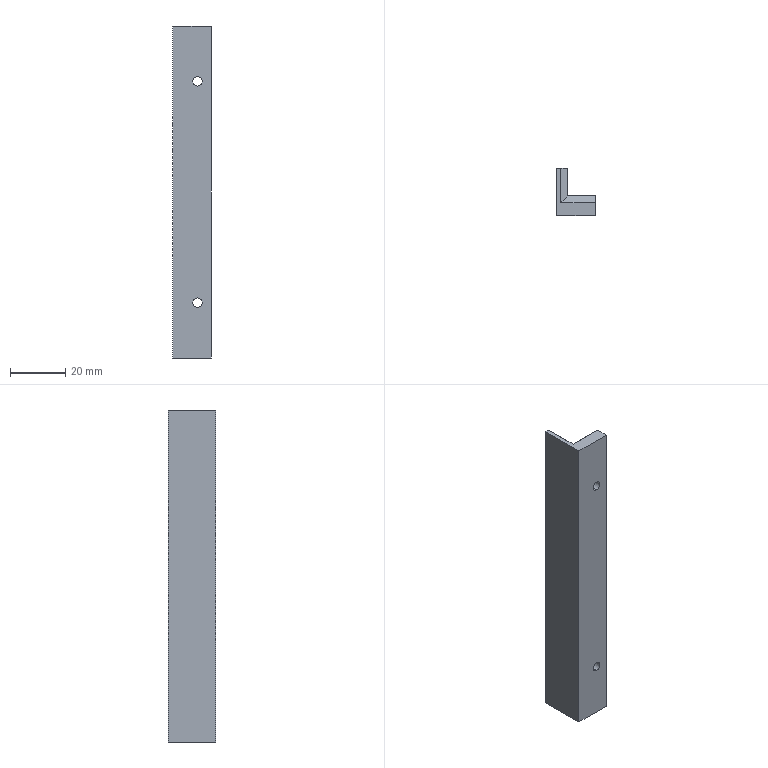Part | NX | features BREP 1 | 1 solid | 20 faces | box 14 x 17 x 120 mm | volume 16235 mm3 | plane 12 | cone 4 | cylinder 4 | commonest cylinder face diameters 3.4 x4
STEP:
#1=CARTESIAN_POINT('',(0.,7.,57.5));
#2=VERTEX_POINT('',#1);
#3=CARTESIAN_POINT('',(0.,4.5,60.));
#4=VERTEX_POINT('',#3);
#5=CARTESIAN_POINT('',(0.,4.5,60.));
#6=DIRECTION('',(0.,-0.7071,0.7071));
#7=VECTOR('',#6,1000.);
#8=LINE('',#5,#7);
#9=EDGE_CURVE('',#2,#4,#8,.T.);
#10=ORIENTED_EDGE('',*,*,#9,.F.);
#11=CARTESIAN_POINT('',(-10.,7.,57.5));
#12=VERTEX_POINT('',#11);
#13=CARTESIAN_POINT('',(-10.,7.,57.5));
#14=DIRECTION('',(1.,0.,0.));
#15=VECTOR('',#14,1000.);
#16=LINE('',#13,#15);
#17=EDGE_CURVE('',#12,#2,#16,.T.);
#18=ORIENTED_EDGE('',*,*,#17,.F.);
#19=CARTESIAN_POINT('',(-12.5,4.5,60.));
#20=VERTEX_POINT('',#19);
#21=CARTESIAN_POINT('',(-8.333,8.667,55.833));
#22=DIRECTION('',(-0.5774,-0.5774,0.5774));
#23=VECTOR('',#22,1000.);
#24=LINE('',#21,#23);
#25=EDGE_CURVE('',#12,#20,#24,.T.);
#26=ORIENTED_EDGE('',*,*,#25,.T.);
#27=CARTESIAN_POINT('',(0.,4.5,60.));
#28=DIRECTION('',(-1.,0.,0.));
#29=VECTOR('',#28,1000.);
#30=LINE('',#27,#29);
#31=EDGE_CURVE('',#4,#20,#30,.T.);
#32=ORIENTED_EDGE('',*,*,#31,.F.);
#33=EDGE_LOOP('',(#10,#18,#26,#32));
#34=FACE_BOUND('',#33,.T.);
#35=CARTESIAN_POINT('',(0.,4.5,60.));
#36=DIRECTION('',(0.,-0.7071,-0.7071));
#37=DIRECTION('',(-1.,0.,0.));
#38=AXIS2_PLACEMENT_3D('',#35,#36,#37);
#39=PLANE('',#38);
#40=ADVANCED_FACE('',(#34),#39,.F.);
#41=CARTESIAN_POINT('',(-12.5,17.,60.));
#42=VERTEX_POINT('',#41);
#43=CARTESIAN_POINT('',(-10.,17.,57.5));
#44=VERTEX_POINT('',#43);
#45=CARTESIAN_POINT('',(-12.5,17.,60.));
#46=DIRECTION('',(0.7071,0.,-0.7071));
#47=VECTOR('',#46,1000.);
#48=LINE('',#45,#47);
#49=EDGE_CURVE('',#42,#44,#48,.T.);
#50=ORIENTED_EDGE('',*,*,#49,.F.);
#51=CARTESIAN_POINT('',(-12.5,0.,60.));
#52=DIRECTION('',(0.,1.,0.));
#53=VECTOR('',#52,1000.);
#54=LINE('',#51,#53);
#55=EDGE_CURVE('',#20,#42,#54,.T.);
#56=ORIENTED_EDGE('',*,*,#55,.F.);
#57=ORIENTED_EDGE('',*,*,#25,.F.);
#58=CARTESIAN_POINT('',(-10.,17.,57.5));
#59=DIRECTION('',(0.,-1.,0.));
#60=VECTOR('',#59,1000.);
#61=LINE('',#58,#60);
#62=EDGE_CURVE('',#44,#12,#61,.T.);
#63=ORIENTED_EDGE('',*,*,#62,.F.);
#64=EDGE_LOOP('',(#50,#56,#57,#63));
#65=FACE_BOUND('',#64,.T.);
#66=CARTESIAN_POINT('',(-12.5,0.,60.));
#67=DIRECTION('',(-0.7071,0.,-0.7071));
#68=DIRECTION('',(0.,1.,0.));
#69=AXIS2_PLACEMENT_3D('',#66,#67,#68);
#70=PLANE('',#69);
#71=ADVANCED_FACE('',(#65),#70,.F.);
#72=CARTESIAN_POINT('',(-10.,7.,-57.5));
#73=VERTEX_POINT('',#72);
#74=CARTESIAN_POINT('',(-12.5,4.5,-60.));
#75=VERTEX_POINT('',#74);
#76=CARTESIAN_POINT('',(-6.667,10.333,-54.167));
#77=DIRECTION('',(-0.5774,-0.5774,-0.5774));
#78=VECTOR('',#77,1000.);
#79=LINE('',#76,#78);
#80=EDGE_CURVE('',#73,#75,#79,.T.);
#81=ORIENTED_EDGE('',*,*,#80,.T.);
#82=CARTESIAN_POINT('',(-12.5,17.,-60.));
#83=VERTEX_POINT('',#82);
#84=CARTESIAN_POINT('',(-12.5,7.,-60.));
#85=DIRECTION('',(0.,-1.,0.));
#86=VECTOR('',#85,1000.);
#87=LINE('',#84,#86);
#88=EDGE_CURVE('',#83,#75,#87,.T.);
#89=ORIENTED_EDGE('',*,*,#88,.F.);
#90=CARTESIAN_POINT('',(-10.,17.,-57.5));
#91=VERTEX_POINT('',#90);
#92=CARTESIAN_POINT('',(-10.,17.,-57.5));
#93=DIRECTION('',(-0.7071,0.,-0.7071));
#94=VECTOR('',#93,1000.);
#95=LINE('',#92,#94);
#96=EDGE_CURVE('',#91,#83,#95,.T.);
#97=ORIENTED_EDGE('',*,*,#96,.F.);
#98=CARTESIAN_POINT('',(-10.,17.,-57.5));
#99=DIRECTION('',(0.,1.,0.));
#100=VECTOR('',#99,1000.);
#101=LINE('',#98,#100);
#102=EDGE_CURVE('',#73,#91,#101,.T.);
#103=ORIENTED_EDGE('',*,*,#102,.F.);
#104=EDGE_LOOP('',(#81,#89,#97,#103));
#105=FACE_BOUND('',#104,.T.);
#106=CARTESIAN_POINT('',(-10.,17.,-57.5));
#107=DIRECTION('',(0.7071,0.,-0.7071));
#108=DIRECTION('',(0.,-1.,0.));
#109=AXIS2_PLACEMENT_3D('',#106,#107,#108);
#110=PLANE('',#109);
#111=ADVANCED_FACE('',(#105),#110,.T.);
#112=CARTESIAN_POINT('',(0.,4.5,-60.));
#113=VERTEX_POINT('',#112);
#114=CARTESIAN_POINT('',(0.,7.,-57.5));
#115=VERTEX_POINT('',#114);
#116=CARTESIAN_POINT('',(0.,7.,-57.5));
#117=DIRECTION('',(0.,0.7071,0.7071));
#118=VECTOR('',#117,1000.);
#119=LINE('',#116,#118);
#120=EDGE_CURVE('',#113,#115,#119,.T.);
#121=ORIENTED_EDGE('',*,*,#120,.F.);
#122=CARTESIAN_POINT('',(0.,4.5,-60.));
#123=DIRECTION('',(1.,0.,0.));
#124=VECTOR('',#123,1000.);
#125=LINE('',#122,#124);
#126=EDGE_CURVE('',#75,#113,#125,.T.);
#127=ORIENTED_EDGE('',*,*,#126,.F.);
#128=ORIENTED_EDGE('',*,*,#80,.F.);
#129=CARTESIAN_POINT('',(-10.,7.,-57.5));
#130=DIRECTION('',(-1.,0.,0.));
#131=VECTOR('',#130,1000.);
#132=LINE('',#129,#131);
#133=EDGE_CURVE('',#115,#73,#132,.T.);
#134=ORIENTED_EDGE('',*,*,#133,.F.);
#135=EDGE_LOOP('',(#121,#127,#128,#134));
#136=FACE_BOUND('',#135,.T.);
#137=CARTESIAN_POINT('',(-10.,7.,-57.5));
#138=DIRECTION('',(0.,0.7071,-0.7071));
#139=DIRECTION('',(1.,0.,0.));
#140=AXIS2_PLACEMENT_3D('',#137,#138,#139);
#141=PLANE('',#140);
#142=ADVANCED_FACE('',(#136),#141,.T.);
#143=CARTESIAN_POINT('',(-5.,7.,-43.75));
#144=VERTEX_POINT('',#143);
#145=CARTESIAN_POINT('',(-5.,4.95,-41.7));
#146=VERTEX_POINT('',#145);
#147=CARTESIAN_POINT('',(-5.,7.,-43.75));
#148=DIRECTION('',(0.,0.7071,-0.7071));
#149=VECTOR('',#148,1000.);
#150=LINE('',#147,#149);
#151=EDGE_CURVE('',#144,#146,#150,.F.);
#152=ORIENTED_EDGE('',*,*,#151,.T.);
#153=CARTESIAN_POINT('',(-5.,4.95,-38.3));
#154=VERTEX_POINT('',#153);
#155=CARTESIAN_POINT('',(-5.,4.95,-40.));
#156=DIRECTION('',(0.,1.,0.));
#157=DIRECTION('',(0.,0.,1.));
#158=AXIS2_PLACEMENT_3D('',#155,#156,#157);
#159=CIRCLE('',#158,1.7);
#160=EDGE_CURVE('',#154,#146,#159,.T.);
#161=ORIENTED_EDGE('',*,*,#160,.F.);
#162=CARTESIAN_POINT('',(-5.,7.,-36.25));
#163=VERTEX_POINT('',#162);
#164=CARTESIAN_POINT('',(-5.,7.,-36.25));
#165=DIRECTION('',(0.,0.7071,0.7071));
#166=VECTOR('',#165,1000.);
#167=LINE('',#164,#166);
#168=EDGE_CURVE('',#163,#154,#167,.F.);
#169=ORIENTED_EDGE('',*,*,#168,.F.);
#170=CARTESIAN_POINT('',(-5.,7.,-40.));
#171=DIRECTION('',(0.,1.,0.));
#172=DIRECTION('',(0.,0.,1.));
#173=AXIS2_PLACEMENT_3D('',#170,#171,#172);
#174=CIRCLE('',#173,3.75);
#175=EDGE_CURVE('',#163,#144,#174,.T.);
#176=ORIENTED_EDGE('',*,*,#175,.T.);
#177=EDGE_LOOP('',(#152,#161,#169,#176));
#178=FACE_BOUND('',#177,.T.);
#179=CARTESIAN_POINT('',(-5.,7.,-40.));
#180=DIRECTION('',(0.,1.,0.));
#181=DIRECTION('',(0.,0.,1.));
#182=AXIS2_PLACEMENT_3D('',#179,#180,#181);
#183=CONICAL_SURFACE('',#182,3.75,0.7854);
#184=ADVANCED_FACE('',(#178),#183,.F.);
#185=CARTESIAN_POINT('',(-5.,0.,-41.7));
#186=VERTEX_POINT('',#185);
#187=CARTESIAN_POINT('',(-5.,7.,-41.7));
#188=DIRECTION('',(0.,1.,0.));
#189=VECTOR('',#188,1000.);
#190=LINE('',#187,#189);
#191=EDGE_CURVE('',#146,#186,#190,.F.);
#192=ORIENTED_EDGE('',*,*,#191,.T.);
#193=CARTESIAN_POINT('',(-5.,0.,-38.3));
#194=VERTEX_POINT('',#193);
#195=CARTESIAN_POINT('',(-5.,0.,-40.));
#196=DIRECTION('',(0.,1.,0.));
#197=DIRECTION('',(-1.,0.,0.));
#198=AXIS2_PLACEMENT_3D('',#195,#196,#197);
#199=CIRCLE('',#198,1.7);
#200=EDGE_CURVE('',#194,#186,#199,.T.);
#201=ORIENTED_EDGE('',*,*,#200,.F.);
#202=CARTESIAN_POINT('',(-5.,7.,-38.3));
#203=DIRECTION('',(0.,1.,0.));
#204=VECTOR('',#203,1000.);
#205=LINE('',#202,#204);
#206=EDGE_CURVE('',#154,#194,#205,.F.);
#207=ORIENTED_EDGE('',*,*,#206,.F.);
#208=ORIENTED_EDGE('',*,*,#160,.T.);
#209=EDGE_LOOP('',(#192,#201,#207,#208));
#210=FACE_BOUND('',#209,.T.);
#211=CARTESIAN_POINT('',(-5.,7.,-40.));
#212=DIRECTION('',(0.,1.,0.));
#213=DIRECTION('',(0.,0.,1.));
#214=AXIS2_PLACEMENT_3D('',#211,#212,#213);
#215=CYLINDRICAL_SURFACE('',#214,1.7);
#216=ADVANCED_FACE('',(#210),#215,.F.);
#217=CARTESIAN_POINT('',(-5.,7.,36.25));
#218=VERTEX_POINT('',#217);
#219=CARTESIAN_POINT('',(-5.,4.95,38.3));
#220=VERTEX_POINT('',#219);
#221=CARTESIAN_POINT('',(-5.,7.,36.25));
#222=DIRECTION('',(0.,0.7071,-0.7071));
#223=VECTOR('',#222,1000.);
#224=LINE('',#221,#223);
#225=EDGE_CURVE('',#218,#220,#224,.F.);
#226=ORIENTED_EDGE('',*,*,#225,.T.);
#227=CARTESIAN_POINT('',(-5.,4.95,41.7));
#228=VERTEX_POINT('',#227);
#229=CARTESIAN_POINT('',(-5.,4.95,40.));
#230=DIRECTION('',(0.,1.,0.));
#231=DIRECTION('',(0.,0.,1.));
#232=AXIS2_PLACEMENT_3D('',#229,#230,#231);
#233=CIRCLE('',#232,1.7);
#234=EDGE_CURVE('',#228,#220,#233,.T.);
#235=ORIENTED_EDGE('',*,*,#234,.F.);
#236=CARTESIAN_POINT('',(-5.,7.,43.75));
#237=VERTEX_POINT('',#236);
#238=CARTESIAN_POINT('',(-5.,7.,43.75));
#239=DIRECTION('',(0.,0.7071,0.7071));
#240=VECTOR('',#239,1000.);
#241=LINE('',#238,#240);
#242=EDGE_CURVE('',#237,#228,#241,.F.);
#243=ORIENTED_EDGE('',*,*,#242,.F.);
#244=CARTESIAN_POINT('',(-5.,7.,40.));
#245=DIRECTION('',(0.,1.,0.));
#246=DIRECTION('',(0.,0.,1.));
#247=AXIS2_PLACEMENT_3D('',#244,#245,#246);
#248=CIRCLE('',#247,3.75);
#249=EDGE_CURVE('',#237,#218,#248,.T.);
#250=ORIENTED_EDGE('',*,*,#249,.T.);
#251=EDGE_LOOP('',(#226,#235,#243,#250));
#252=FACE_BOUND('',#251,.T.);
#253=CARTESIAN_POINT('',(-5.,7.,40.));
#254=DIRECTION('',(0.,1.,0.));
#255=DIRECTION('',(0.,0.,1.));
#256=AXIS2_PLACEMENT_3D('',#253,#254,#255);
#257=CONICAL_SURFACE('',#256,3.75,0.7854);
#258=ADVANCED_FACE('',(#252),#257,.F.);
#259=CARTESIAN_POINT('',(-5.,0.,38.3));
#260=VERTEX_POINT('',#259);
#261=CARTESIAN_POINT('',(-5.,7.,38.3));
#262=DIRECTION('',(0.,1.,0.));
#263=VECTOR('',#262,1000.);
#264=LINE('',#261,#263);
#265=EDGE_CURVE('',#220,#260,#264,.F.);
#266=ORIENTED_EDGE('',*,*,#265,.T.);
#267=CARTESIAN_POINT('',(-5.,0.,41.7));
#268=VERTEX_POINT('',#267);
#269=CARTESIAN_POINT('',(-5.,0.,40.));
#270=DIRECTION('',(0.,1.,0.));
#271=DIRECTION('',(-1.,0.,0.));
#272=AXIS2_PLACEMENT_3D('',#269,#270,#271);
#273=CIRCLE('',#272,1.7);
#274=EDGE_CURVE('',#268,#260,#273,.T.);
#275=ORIENTED_EDGE('',*,*,#274,.F.);
#276=CARTESIAN_POINT('',(-5.,7.,41.7));
#277=DIRECTION('',(0.,1.,0.));
#278=VECTOR('',#277,1000.);
#279=LINE('',#276,#278);
#280=EDGE_CURVE('',#228,#268,#279,.F.);
#281=ORIENTED_EDGE('',*,*,#280,.F.);
#282=ORIENTED_EDGE('',*,*,#234,.T.);
#283=EDGE_LOOP('',(#266,#275,#281,#282));
#284=FACE_BOUND('',#283,.T.);
#285=CARTESIAN_POINT('',(-5.,7.,40.));
#286=DIRECTION('',(0.,1.,0.));
#287=DIRECTION('',(0.,0.,1.));
#288=AXIS2_PLACEMENT_3D('',#285,#286,#287);
#289=CYLINDRICAL_SURFACE('',#288,1.7);
#290=ADVANCED_FACE('',(#284),#289,.F.);
#291=CARTESIAN_POINT('',(-14.,17.,-60.));
#292=VERTEX_POINT('',#291);
#293=CARTESIAN_POINT('',(-14.,17.,-60.));
#294=DIRECTION('',(-1.,0.,0.));
#295=VECTOR('',#294,1000.);
#296=LINE('',#293,#295);
#297=EDGE_CURVE('',#83,#292,#296,.T.);
#298=ORIENTED_EDGE('',*,*,#297,.F.);
#299=ORIENTED_EDGE('',*,*,#88,.T.);
#300=ORIENTED_EDGE('',*,*,#126,.T.);
#301=CARTESIAN_POINT('',(0.,0.,-60.));
#302=VERTEX_POINT('',#301);
#303=CARTESIAN_POINT('',(0.,7.,-60.));
#304=DIRECTION('',(0.,1.,0.));
#305=VECTOR('',#304,1000.);
#306=LINE('',#303,#305);
#307=EDGE_CURVE('',#302,#113,#306,.T.);
#308=ORIENTED_EDGE('',*,*,#307,.F.);
#309=CARTESIAN_POINT('',(-14.,0.,-60.));
#310=VERTEX_POINT('',#309);
#311=CARTESIAN_POINT('',(0.,0.,-60.));
#312=DIRECTION('',(1.,0.,0.));
#313=VECTOR('',#312,1000.);
#314=LINE('',#311,#313);
#315=EDGE_CURVE('',#310,#302,#314,.T.);
#316=ORIENTED_EDGE('',*,*,#315,.F.);
#317=CARTESIAN_POINT('',(-14.,0.,-60.));
#318=DIRECTION('',(0.,-1.,0.));
#319=VECTOR('',#318,1000.);
#320=LINE('',#317,#319);
#321=EDGE_CURVE('',#292,#310,#320,.T.);
#322=ORIENTED_EDGE('',*,*,#321,.F.);
#323=EDGE_LOOP('',(#298,#299,#300,#308,#316,#322));
#324=FACE_BOUND('',#323,.T.);
#325=CARTESIAN_POINT('',(0.,0.,-60.));
#326=DIRECTION('',(0.,0.,-1.));
#327=DIRECTION('',(-1.,0.,0.));
#328=AXIS2_PLACEMENT_3D('',#325,#326,#327);
#329=PLANE('',#328);
#330=ADVANCED_FACE('',(#324),#329,.T.);
#331=CARTESIAN_POINT('',(0.,0.,60.));
#332=VERTEX_POINT('',#331);
#333=CARTESIAN_POINT('',(0.,7.,60.));
#334=DIRECTION('',(0.,1.,0.));
#335=VECTOR('',#334,1000.);
#336=LINE('',#333,#335);
#337=EDGE_CURVE('',#332,#4,#336,.T.);
#338=ORIENTED_EDGE('',*,*,#337,.T.);
#339=ORIENTED_EDGE('',*,*,#31,.T.);
#340=ORIENTED_EDGE('',*,*,#55,.T.);
#341=CARTESIAN_POINT('',(-14.,17.,60.));
#342=VERTEX_POINT('',#341);
#343=CARTESIAN_POINT('',(-14.,17.,60.));
#344=DIRECTION('',(-1.,0.,0.));
#345=VECTOR('',#344,1000.);
#346=LINE('',#343,#345);
#347=EDGE_CURVE('',#42,#342,#346,.T.);
#348=ORIENTED_EDGE('',*,*,#347,.T.);
#349=CARTESIAN_POINT('',(-14.,0.,60.));
#350=VERTEX_POINT('',#349);
#351=CARTESIAN_POINT('',(-14.,0.,60.));
#352=DIRECTION('',(0.,-1.,0.));
#353=VECTOR('',#352,1000.);
#354=LINE('',#351,#353);
#355=EDGE_CURVE('',#342,#350,#354,.T.);
#356=ORIENTED_EDGE('',*,*,#355,.T.);
#357=CARTESIAN_POINT('',(0.,0.,60.));
#358=DIRECTION('',(1.,0.,0.));
#359=VECTOR('',#358,1000.);
#360=LINE('',#357,#359);
#361=EDGE_CURVE('',#350,#332,#360,.T.);
#362=ORIENTED_EDGE('',*,*,#361,.T.);
#363=EDGE_LOOP('',(#338,#339,#340,#348,#356,#362));
#364=FACE_BOUND('',#363,.T.);
#365=CARTESIAN_POINT('',(0.,0.,60.));
#366=DIRECTION('',(0.,0.,-1.));
#367=DIRECTION('',(-1.,0.,0.));
#368=AXIS2_PLACEMENT_3D('',#365,#366,#367);
#369=PLANE('',#368);
#370=ADVANCED_FACE('',(#364),#369,.F.);
#371=ORIENTED_EDGE('',*,*,#315,.T.);
#372=CARTESIAN_POINT('',(0.,0.,60.));
#373=DIRECTION('',(0.,0.,-1.));
#374=VECTOR('',#373,1000.);
#375=LINE('',#372,#374);
#376=EDGE_CURVE('',#332,#302,#375,.T.);
#377=ORIENTED_EDGE('',*,*,#376,.F.);
#378=ORIENTED_EDGE('',*,*,#361,.F.);
#379=CARTESIAN_POINT('',(-14.,0.,60.));
#380=DIRECTION('',(0.,0.,-1.));
#381=VECTOR('',#380,1000.);
#382=LINE('',#379,#381);
#383=EDGE_CURVE('',#350,#310,#382,.T.);
#384=ORIENTED_EDGE('',*,*,#383,.T.);
#385=EDGE_LOOP('',(#371,#377,#378,#384));
#386=FACE_BOUND('',#385,.T.);
#387=ORIENTED_EDGE('',*,*,#274,.T.);
#388=CARTESIAN_POINT('',(-5.,0.,40.));
#389=DIRECTION('',(0.,1.,0.));
#390=DIRECTION('',(-1.,0.,0.));
#391=AXIS2_PLACEMENT_3D('',#388,#389,#390);
#392=CIRCLE('',#391,1.7);
#393=EDGE_CURVE('',#260,#268,#392,.T.);
#394=ORIENTED_EDGE('',*,*,#393,.T.);
#395=EDGE_LOOP('',(#387,#394));
#396=FACE_BOUND('',#395,.T.);
#397=ORIENTED_EDGE('',*,*,#200,.T.);
#398=CARTESIAN_POINT('',(-5.,0.,-40.));
#399=DIRECTION('',(0.,1.,0.));
#400=DIRECTION('',(-1.,0.,0.));
#401=AXIS2_PLACEMENT_3D('',#398,#399,#400);
#402=CIRCLE('',#401,1.7);
#403=EDGE_CURVE('',#186,#194,#402,.T.);
#404=ORIENTED_EDGE('',*,*,#403,.T.);
#405=EDGE_LOOP('',(#397,#404));
#406=FACE_BOUND('',#405,.T.);
#407=CARTESIAN_POINT('',(0.,0.,60.));
#408=DIRECTION('',(0.,1.,0.));
#409=DIRECTION('',(-1.,0.,0.));
#410=AXIS2_PLACEMENT_3D('',#407,#408,#409);
#411=PLANE('',#410);
#412=ADVANCED_FACE('',(#386,#396,#406),#411,.F.);
#413=ORIENTED_EDGE('',*,*,#321,.T.);
#414=ORIENTED_EDGE('',*,*,#383,.F.);
#415=ORIENTED_EDGE('',*,*,#355,.F.);
#416=CARTESIAN_POINT('',(-14.,17.,60.));
#417=DIRECTION('',(0.,0.,-1.));
#418=VECTOR('',#417,1000.);
#419=LINE('',#416,#418);
#420=EDGE_CURVE('',#342,#292,#419,.T.);
#421=ORIENTED_EDGE('',*,*,#420,.T.);
#422=EDGE_LOOP('',(#413,#414,#415,#421));
#423=FACE_BOUND('',#422,.T.);
#424=CARTESIAN_POINT('',(-14.,0.,60.));
#425=DIRECTION('',(1.,0.,0.));
#426=DIRECTION('',(0.,1.,0.));
#427=AXIS2_PLACEMENT_3D('',#424,#425,#426);
#428=PLANE('',#427);
#429=ADVANCED_FACE('',(#423),#428,.F.);
#430=CARTESIAN_POINT('',(-10.,17.,60.));
#431=DIRECTION('',(0.,0.,-1.));
#432=VECTOR('',#431,1000.);
#433=LINE('',#430,#432);
#434=EDGE_CURVE('',#44,#91,#433,.T.);
#435=ORIENTED_EDGE('',*,*,#434,.T.);
#436=ORIENTED_EDGE('',*,*,#96,.T.);
#437=ORIENTED_EDGE('',*,*,#297,.T.);
#438=ORIENTED_EDGE('',*,*,#420,.F.);
#439=ORIENTED_EDGE('',*,*,#347,.F.);
#440=ORIENTED_EDGE('',*,*,#49,.T.);
#441=EDGE_LOOP('',(#435,#436,#437,#438,#439,#440));
#442=FACE_BOUND('',#441,.T.);
#443=CARTESIAN_POINT('',(-14.,17.,60.));
#444=DIRECTION('',(0.,-1.,0.));
#445=DIRECTION('',(1.,0.,0.));
#446=AXIS2_PLACEMENT_3D('',#443,#444,#445);
#447=PLANE('',#446);
#448=ADVANCED_FACE('',(#442),#447,.F.);
#449=CARTESIAN_POINT('',(-10.,7.,60.));
#450=DIRECTION('',(0.,0.,-1.));
#451=VECTOR('',#450,1000.);
#452=LINE('',#449,#451);
#453=EDGE_CURVE('',#12,#73,#452,.T.);
#454=ORIENTED_EDGE('',*,*,#453,.T.);
#455=ORIENTED_EDGE('',*,*,#102,.T.);
#456=ORIENTED_EDGE('',*,*,#434,.F.);
#457=ORIENTED_EDGE('',*,*,#62,.T.);
#458=EDGE_LOOP('',(#454,#455,#456,#457));
#459=FACE_BOUND('',#458,.T.);
#460=CARTESIAN_POINT('',(-10.,17.,60.));
#461=DIRECTION('',(-1.,0.,0.));
#462=DIRECTION('',(0.,-1.,0.));
#463=AXIS2_PLACEMENT_3D('',#460,#461,#462);
#464=PLANE('',#463);
#465=ADVANCED_FACE('',(#459),#464,.F.);
#466=CARTESIAN_POINT('',(0.,7.,60.));
#467=DIRECTION('',(0.,0.,-1.));
#468=VECTOR('',#467,1000.);
#469=LINE('',#466,#468);
#470=EDGE_CURVE('',#2,#115,#469,.T.);
#471=ORIENTED_EDGE('',*,*,#470,.T.);
#472=ORIENTED_EDGE('',*,*,#133,.T.);
#473=ORIENTED_EDGE('',*,*,#453,.F.);
#474=ORIENTED_EDGE('',*,*,#17,.T.);
#475=EDGE_LOOP('',(#471,#472,#473,#474));
#476=FACE_BOUND('',#475,.T.);
#477=ORIENTED_EDGE('',*,*,#249,.F.);
#478=CARTESIAN_POINT('',(-5.,7.,40.));
#479=DIRECTION('',(0.,1.,0.));
#480=DIRECTION('',(0.,0.,1.));
#481=AXIS2_PLACEMENT_3D('',#478,#479,#480);
#482=CIRCLE('',#481,3.75);
#483=EDGE_CURVE('',#218,#237,#482,.T.);
#484=ORIENTED_EDGE('',*,*,#483,.F.);
#485=EDGE_LOOP('',(#477,#484));
#486=FACE_BOUND('',#485,.T.);
#487=ORIENTED_EDGE('',*,*,#175,.F.);
#488=CARTESIAN_POINT('',(-5.,7.,-40.));
#489=DIRECTION('',(0.,1.,0.));
#490=DIRECTION('',(0.,0.,1.));
#491=AXIS2_PLACEMENT_3D('',#488,#489,#490);
#492=CIRCLE('',#491,3.75);
#493=EDGE_CURVE('',#144,#163,#492,.T.);
#494=ORIENTED_EDGE('',*,*,#493,.F.);
#495=EDGE_LOOP('',(#487,#494));
#496=FACE_BOUND('',#495,.T.);
#497=CARTESIAN_POINT('',(-10.,7.,60.));
#498=DIRECTION('',(0.,-1.,0.));
#499=DIRECTION('',(0.,0.,-1.));
#500=AXIS2_PLACEMENT_3D('',#497,#498,#499);
#501=PLANE('',#500);
#502=ADVANCED_FACE('',(#476,#486,#496),#501,.F.);
#503=ORIENTED_EDGE('',*,*,#307,.T.);
#504=ORIENTED_EDGE('',*,*,#120,.T.);
#505=ORIENTED_EDGE('',*,*,#470,.F.);
#506=ORIENTED_EDGE('',*,*,#9,.T.);
#507=ORIENTED_EDGE('',*,*,#337,.F.);
#508=ORIENTED_EDGE('',*,*,#376,.T.);
#509=EDGE_LOOP('',(#503,#504,#505,#506,#507,#508));
#510=FACE_BOUND('',#509,.T.);
#511=CARTESIAN_POINT('',(0.,7.,60.));
#512=DIRECTION('',(-1.,0.,0.));
#513=DIRECTION('',(0.,-1.,0.));
#514=AXIS2_PLACEMENT_3D('',#511,#512,#513);
#515=PLANE('',#514);
#516=ADVANCED_FACE('',(#510),#515,.F.);
#517=ORIENTED_EDGE('',*,*,#393,.F.);
#518=ORIENTED_EDGE('',*,*,#265,.F.);
#519=CARTESIAN_POINT('',(-5.,4.95,40.));
#520=DIRECTION('',(0.,1.,0.));
#521=DIRECTION('',(0.,0.,1.));
#522=AXIS2_PLACEMENT_3D('',#519,#520,#521);
#523=CIRCLE('',#522,1.7);
#524=EDGE_CURVE('',#220,#228,#523,.T.);
#525=ORIENTED_EDGE('',*,*,#524,.T.);
#526=ORIENTED_EDGE('',*,*,#280,.T.);
#527=EDGE_LOOP('',(#517,#518,#525,#526));
#528=FACE_BOUND('',#527,.T.);
#529=CARTESIAN_POINT('',(-5.,7.,40.));
#530=DIRECTION('',(0.,1.,0.));
#531=DIRECTION('',(0.,0.,1.));
#532=AXIS2_PLACEMENT_3D('',#529,#530,#531);
#533=CYLINDRICAL_SURFACE('',#532,1.7);
#534=ADVANCED_FACE('',(#528),#533,.F.);
#535=ORIENTED_EDGE('',*,*,#524,.F.);
#536=ORIENTED_EDGE('',*,*,#225,.F.);
#537=ORIENTED_EDGE('',*,*,#483,.T.);
#538=ORIENTED_EDGE('',*,*,#242,.T.);
#539=EDGE_LOOP('',(#535,#536,#537,#538));
#540=FACE_BOUND('',#539,.T.);
#541=CARTESIAN_POINT('',(-5.,7.,40.));
#542=DIRECTION('',(0.,1.,0.));
#543=DIRECTION('',(0.,0.,1.));
#544=AXIS2_PLACEMENT_3D('',#541,#542,#543);
#545=CONICAL_SURFACE('',#544,3.75,0.7854);
#546=ADVANCED_FACE('',(#540),#545,.F.);
#547=ORIENTED_EDGE('',*,*,#403,.F.);
#548=ORIENTED_EDGE('',*,*,#191,.F.);
#549=CARTESIAN_POINT('',(-5.,4.95,-40.));
#550=DIRECTION('',(0.,1.,0.));
#551=DIRECTION('',(0.,0.,1.));
#552=AXIS2_PLACEMENT_3D('',#549,#550,#551);
#553=CIRCLE('',#552,1.7);
#554=EDGE_CURVE('',#146,#154,#553,.T.);
#555=ORIENTED_EDGE('',*,*,#554,.T.);
#556=ORIENTED_EDGE('',*,*,#206,.T.);
#557=EDGE_LOOP('',(#547,#548,#555,#556));
#558=FACE_BOUND('',#557,.T.);
#559=CARTESIAN_POINT('',(-5.,7.,-40.));
#560=DIRECTION('',(0.,1.,0.));
#561=DIRECTION('',(0.,0.,1.));
#562=AXIS2_PLACEMENT_3D('',#559,#560,#561);
#563=CYLINDRICAL_SURFACE('',#562,1.7);
#564=ADVANCED_FACE('',(#558),#563,.F.);
#565=ORIENTED_EDGE('',*,*,#554,.F.);
#566=ORIENTED_EDGE('',*,*,#151,.F.);
#567=ORIENTED_EDGE('',*,*,#493,.T.);
#568=ORIENTED_EDGE('',*,*,#168,.T.);
#569=EDGE_LOOP('',(#565,#566,#567,#568));
#570=FACE_BOUND('',#569,.T.);
#571=CARTESIAN_POINT('',(-5.,7.,-40.));
#572=DIRECTION('',(0.,1.,0.));
#573=DIRECTION('',(0.,0.,1.));
#574=AXIS2_PLACEMENT_3D('',#571,#572,#573);
#575=CONICAL_SURFACE('',#574,3.75,0.7854);
#576=ADVANCED_FACE('',(#570),#575,.F.);
#577=CLOSED_SHELL('',(#40,#71,#111,#142,#184,#216,#258,#290,#330,#370,#412,#429,#448,#465,#502,#516,#534,#546,#564,#576));
#578=MANIFOLD_SOLID_BREP('',#577);
#579=(LENGTH_UNIT()NAMED_UNIT(*)SI_UNIT(.MILLI.,.METRE.));
#580=UNCERTAINTY_MEASURE_WITH_UNIT(LENGTH_MEASURE(0.00001),#579,'','');
#581=(NAMED_UNIT(*)PLANE_ANGLE_UNIT()SI_UNIT($,.RADIAN.));
#582=(NAMED_UNIT(*)SI_UNIT($,.STERADIAN.)SOLID_ANGLE_UNIT());
#583=(GEOMETRIC_REPRESENTATION_CONTEXT(3)GLOBAL_UNCERTAINTY_ASSIGNED_CONTEXT((#580))GLOBAL_UNIT_ASSIGNED_CONTEXT((#579,#581,#582))REPRESENTATION_CONTEXT('',''));
#584=ADVANCED_BREP_SHAPE_REPRESENTATION('',(#578),#583);